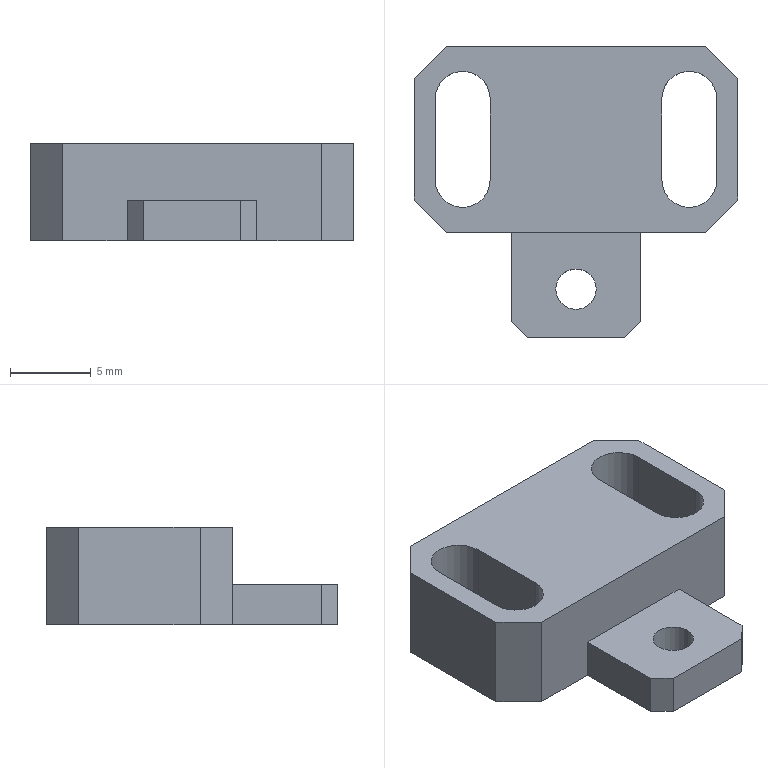Part | SolidWorks | features HoleWzd 3, Chamfer 2, ICE 2, Extrusion 1 | 1 solid | 26 faces | box 20 x 18 x 6 mm | volume 1134 mm3 | plane 20 | cylinder 6 | commonest cylinder face diameters 3.4 x4 2.5 x2
STEP:
#1=CARTESIAN_POINT('',(-1.25,-6.,0.));
#2=VERTEX_POINT('',#1);
#3=CARTESIAN_POINT('',(1.25,-6.,0.));
#4=VERTEX_POINT('',#3);
#5=CARTESIAN_POINT('',(0.,-6.,0.));
#6=DIRECTION('',(0.,0.,1.));
#7=DIRECTION('',(1.,0.,0.));
#8=AXIS2_PLACEMENT_3D('',#5,#6,#7);
#9=CIRCLE('',#8,1.25);
#10=EDGE_CURVE('',#2,#4,#9,.T.);
#11=ORIENTED_EDGE('',*,*,#10,.F.);
#12=CARTESIAN_POINT('',(-1.25,-6.,2.5));
#13=VERTEX_POINT('',#12);
#14=CARTESIAN_POINT('',(-1.25,-6.,6.));
#15=DIRECTION('',(0.,0.,1.));
#16=VECTOR('',#15,1000.);
#17=LINE('',#14,#16);
#18=EDGE_CURVE('',#2,#13,#17,.T.);
#19=ORIENTED_EDGE('',*,*,#18,.T.);
#20=CARTESIAN_POINT('',(1.25,-6.,2.5));
#21=VERTEX_POINT('',#20);
#22=CARTESIAN_POINT('',(0.,-6.,2.5));
#23=DIRECTION('',(0.,0.,-1.));
#24=DIRECTION('',(1.,0.,0.));
#25=AXIS2_PLACEMENT_3D('',#22,#23,#24);
#26=CIRCLE('',#25,1.25);
#27=EDGE_CURVE('',#21,#13,#26,.T.);
#28=ORIENTED_EDGE('',*,*,#27,.F.);
#29=CARTESIAN_POINT('',(1.25,-6.,6.));
#30=DIRECTION('',(0.,0.,1.));
#31=VECTOR('',#30,1000.);
#32=LINE('',#29,#31);
#33=EDGE_CURVE('',#4,#21,#32,.T.);
#34=ORIENTED_EDGE('',*,*,#33,.F.);
#35=EDGE_LOOP('',(#11,#19,#28,#34));
#36=FACE_OUTER_BOUND('',#35,.T.);
#37=CARTESIAN_POINT('',(0.,-6.,6.));
#38=DIRECTION('',(0.,0.,1.));
#39=DIRECTION('',(1.,0.,0.));
#40=AXIS2_PLACEMENT_3D('',#37,#38,#39);
#41=CYLINDRICAL_SURFACE('',#40,1.25);
#42=ADVANCED_FACE('',(#36),#41,.F.);
#43=CARTESIAN_POINT('',(-4.,-2.5,0.));
#44=VERTEX_POINT('',#43);
#45=CARTESIAN_POINT('',(-4.,-8.,0.));
#46=VERTEX_POINT('',#45);
#47=CARTESIAN_POINT('',(-4.,9.,0.));
#48=DIRECTION('',(0.,-1.,0.));
#49=VECTOR('',#48,1000.);
#50=LINE('',#47,#49);
#51=EDGE_CURVE('',#44,#46,#50,.T.);
#52=ORIENTED_EDGE('',*,*,#51,.T.);
#53=CARTESIAN_POINT('',(-4.,-8.,2.5));
#54=VERTEX_POINT('',#53);
#55=CARTESIAN_POINT('',(-4.,-8.,6.));
#56=DIRECTION('',(0.,0.,1.));
#57=VECTOR('',#56,1000.);
#58=LINE('',#55,#57);
#59=EDGE_CURVE('',#46,#54,#58,.T.);
#60=ORIENTED_EDGE('',*,*,#59,.T.);
#61=CARTESIAN_POINT('',(-4.,-2.5,2.5));
#62=VERTEX_POINT('',#61);
#63=CARTESIAN_POINT('',(-4.,-9.,2.5));
#64=DIRECTION('',(0.,1.,0.));
#65=VECTOR('',#64,1000.);
#66=LINE('',#63,#65);
#67=EDGE_CURVE('',#54,#62,#66,.T.);
#68=ORIENTED_EDGE('',*,*,#67,.T.);
#69=CARTESIAN_POINT('',(-4.,-2.5,-12.971));
#70=DIRECTION('',(0.,0.,1.));
#71=VECTOR('',#70,1000.);
#72=LINE('',#69,#71);
#73=EDGE_CURVE('',#44,#62,#72,.T.);
#74=ORIENTED_EDGE('',*,*,#73,.F.);
#75=EDGE_LOOP('',(#52,#60,#68,#74));
#76=FACE_OUTER_BOUND('',#75,.T.);
#77=CARTESIAN_POINT('',(-4.,9.,6.));
#78=DIRECTION('',(1.,0.,0.));
#79=DIRECTION('',(0.,1.,0.));
#80=AXIS2_PLACEMENT_3D('',#77,#78,#79);
#81=PLANE('',#80);
#82=ADVANCED_FACE('',(#76),#81,.F.);
#83=CARTESIAN_POINT('',(3.,-9.,2.5));
#84=VERTEX_POINT('',#83);
#85=CARTESIAN_POINT('',(-3.,-9.,2.5));
#86=VERTEX_POINT('',#85);
#87=CARTESIAN_POINT('',(-4.,-9.,2.5));
#88=DIRECTION('',(-1.,0.,0.));
#89=VECTOR('',#88,1000.);
#90=LINE('',#87,#89);
#91=EDGE_CURVE('',#84,#86,#90,.T.);
#92=ORIENTED_EDGE('',*,*,#91,.T.);
#93=CARTESIAN_POINT('',(-3.,-9.,0.));
#94=VERTEX_POINT('',#93);
#95=CARTESIAN_POINT('',(-3.,-9.,6.));
#96=DIRECTION('',(0.,0.,-1.));
#97=VECTOR('',#96,1000.);
#98=LINE('',#95,#97);
#99=EDGE_CURVE('',#86,#94,#98,.T.);
#100=ORIENTED_EDGE('',*,*,#99,.T.);
#101=CARTESIAN_POINT('',(3.,-9.,0.));
#102=VERTEX_POINT('',#101);
#103=CARTESIAN_POINT('',(-4.,-9.,0.));
#104=DIRECTION('',(1.,0.,0.));
#105=VECTOR('',#104,1000.);
#106=LINE('',#103,#105);
#107=EDGE_CURVE('',#94,#102,#106,.T.);
#108=ORIENTED_EDGE('',*,*,#107,.T.);
#109=CARTESIAN_POINT('',(3.,-9.,6.));
#110=DIRECTION('',(0.,0.,1.));
#111=VECTOR('',#110,1000.);
#112=LINE('',#109,#111);
#113=EDGE_CURVE('',#102,#84,#112,.T.);
#114=ORIENTED_EDGE('',*,*,#113,.T.);
#115=EDGE_LOOP('',(#92,#100,#108,#114));
#116=FACE_OUTER_BOUND('',#115,.T.);
#117=CARTESIAN_POINT('',(-4.,-9.,6.));
#118=DIRECTION('',(0.,1.,0.));
#119=DIRECTION('',(0.,0.,1.));
#120=AXIS2_PLACEMENT_3D('',#117,#118,#119);
#121=PLANE('',#120);
#122=ADVANCED_FACE('',(#116),#121,.F.);
#123=ORIENTED_EDGE('',*,*,#18,.F.);
#124=CARTESIAN_POINT('',(0.,-6.,0.));
#125=DIRECTION('',(0.,0.,1.));
#126=DIRECTION('',(1.,0.,0.));
#127=AXIS2_PLACEMENT_3D('',#124,#125,#126);
#128=CIRCLE('',#127,1.25);
#129=EDGE_CURVE('',#4,#2,#128,.T.);
#130=ORIENTED_EDGE('',*,*,#129,.F.);
#131=ORIENTED_EDGE('',*,*,#33,.T.);
#132=CARTESIAN_POINT('',(0.,-6.,2.5));
#133=DIRECTION('',(0.,0.,-1.));
#134=DIRECTION('',(1.,0.,0.));
#135=AXIS2_PLACEMENT_3D('',#132,#133,#134);
#136=CIRCLE('',#135,1.25);
#137=EDGE_CURVE('',#13,#21,#136,.T.);
#138=ORIENTED_EDGE('',*,*,#137,.F.);
#139=EDGE_LOOP('',(#123,#130,#131,#138));
#140=FACE_OUTER_BOUND('',#139,.T.);
#141=CARTESIAN_POINT('',(0.,-6.,6.));
#142=DIRECTION('',(0.,0.,1.));
#143=DIRECTION('',(1.,0.,0.));
#144=AXIS2_PLACEMENT_3D('',#141,#142,#143);
#145=CYLINDRICAL_SURFACE('',#144,1.25);
#146=ADVANCED_FACE('',(#140),#145,.F.);
#147=CARTESIAN_POINT('',(4.,-2.5,2.5));
#148=VERTEX_POINT('',#147);
#149=CARTESIAN_POINT('',(4.,-8.,2.5));
#150=VERTEX_POINT('',#149);
#151=CARTESIAN_POINT('',(4.,-9.,2.5));
#152=DIRECTION('',(0.,-1.,0.));
#153=VECTOR('',#152,1000.);
#154=LINE('',#151,#153);
#155=EDGE_CURVE('',#148,#150,#154,.T.);
#156=ORIENTED_EDGE('',*,*,#155,.T.);
#157=CARTESIAN_POINT('',(4.,-8.,0.));
#158=VERTEX_POINT('',#157);
#159=CARTESIAN_POINT('',(4.,-8.,6.));
#160=DIRECTION('',(0.,0.,-1.));
#161=VECTOR('',#160,1000.);
#162=LINE('',#159,#161);
#163=EDGE_CURVE('',#150,#158,#162,.T.);
#164=ORIENTED_EDGE('',*,*,#163,.T.);
#165=CARTESIAN_POINT('',(4.,-2.5,0.));
#166=VERTEX_POINT('',#165);
#167=CARTESIAN_POINT('',(4.,9.,0.));
#168=DIRECTION('',(0.,1.,0.));
#169=VECTOR('',#168,1000.);
#170=LINE('',#167,#169);
#171=EDGE_CURVE('',#158,#166,#170,.T.);
#172=ORIENTED_EDGE('',*,*,#171,.T.);
#173=CARTESIAN_POINT('',(4.,-2.5,-12.971));
#174=DIRECTION('',(0.,0.,1.));
#175=VECTOR('',#174,1000.);
#176=LINE('',#173,#175);
#177=EDGE_CURVE('',#166,#148,#176,.T.);
#178=ORIENTED_EDGE('',*,*,#177,.T.);
#179=EDGE_LOOP('',(#156,#164,#172,#178));
#180=FACE_OUTER_BOUND('',#179,.T.);
#181=CARTESIAN_POINT('',(4.,9.,6.));
#182=DIRECTION('',(-1.,0.,0.));
#183=DIRECTION('',(0.,-1.,0.));
#184=AXIS2_PLACEMENT_3D('',#181,#182,#183);
#185=PLANE('',#184);
#186=ADVANCED_FACE('',(#180),#185,.F.);
#187=CARTESIAN_POINT('',(8.,9.,6.));
#188=VERTEX_POINT('',#187);
#189=CARTESIAN_POINT('',(-8.,9.,6.));
#190=VERTEX_POINT('',#189);
#191=CARTESIAN_POINT('',(-4.,9.,6.));
#192=DIRECTION('',(-1.,0.,0.));
#193=VECTOR('',#192,1000.);
#194=LINE('',#191,#193);
#195=EDGE_CURVE('',#188,#190,#194,.T.);
#196=ORIENTED_EDGE('',*,*,#195,.F.);
#197=CARTESIAN_POINT('',(8.,9.,0.));
#198=VERTEX_POINT('',#197);
#199=CARTESIAN_POINT('',(8.,9.,0.));
#200=DIRECTION('',(0.,0.,-1.));
#201=VECTOR('',#200,1000.);
#202=LINE('',#199,#201);
#203=EDGE_CURVE('',#188,#198,#202,.T.);
#204=ORIENTED_EDGE('',*,*,#203,.T.);
#205=CARTESIAN_POINT('',(-8.,9.,0.));
#206=VERTEX_POINT('',#205);
#207=CARTESIAN_POINT('',(-4.,9.,0.));
#208=DIRECTION('',(-1.,0.,0.));
#209=VECTOR('',#208,1000.);
#210=LINE('',#207,#209);
#211=EDGE_CURVE('',#198,#206,#210,.T.);
#212=ORIENTED_EDGE('',*,*,#211,.T.);
#213=CARTESIAN_POINT('',(-8.,9.,6.));
#214=DIRECTION('',(0.,0.,1.));
#215=VECTOR('',#214,1000.);
#216=LINE('',#213,#215);
#217=EDGE_CURVE('',#206,#190,#216,.T.);
#218=ORIENTED_EDGE('',*,*,#217,.T.);
#219=EDGE_LOOP('',(#196,#204,#212,#218));
#220=FACE_OUTER_BOUND('',#219,.T.);
#221=CARTESIAN_POINT('',(-4.,9.,6.));
#222=DIRECTION('',(0.,-1.,0.));
#223=DIRECTION('',(0.,0.,-1.));
#224=AXIS2_PLACEMENT_3D('',#221,#222,#223);
#225=PLANE('',#224);
#226=ADVANCED_FACE('',(#220),#225,.F.);
#227=CARTESIAN_POINT('',(-5.3,5.75,6.));
#228=VERTEX_POINT('',#227);
#229=CARTESIAN_POINT('',(-8.7,5.75,6.));
#230=VERTEX_POINT('',#229);
#231=CARTESIAN_POINT('',(-7.,5.75,6.));
#232=DIRECTION('',(0.,0.,1.));
#233=DIRECTION('',(1.,0.,0.));
#234=AXIS2_PLACEMENT_3D('',#231,#232,#233);
#235=CIRCLE('',#234,1.7);
#236=EDGE_CURVE('',#228,#230,#235,.T.);
#237=ORIENTED_EDGE('',*,*,#236,.F.);
#238=CARTESIAN_POINT('',(-5.3,0.75,6.));
#239=VERTEX_POINT('',#238);
#240=CARTESIAN_POINT('',(-5.3,0.75,6.));
#241=DIRECTION('',(0.,1.,0.));
#242=VECTOR('',#241,1000.);
#243=LINE('',#240,#242);
#244=EDGE_CURVE('',#239,#228,#243,.T.);
#245=ORIENTED_EDGE('',*,*,#244,.F.);
#246=CARTESIAN_POINT('',(-8.7,0.75,6.));
#247=VERTEX_POINT('',#246);
#248=CARTESIAN_POINT('',(-7.,0.75,6.));
#249=DIRECTION('',(0.,0.,1.));
#250=DIRECTION('',(1.,0.,0.));
#251=AXIS2_PLACEMENT_3D('',#248,#249,#250);
#252=CIRCLE('',#251,1.7);
#253=EDGE_CURVE('',#247,#239,#252,.T.);
#254=ORIENTED_EDGE('',*,*,#253,.F.);
#255=CARTESIAN_POINT('',(-8.7,0.75,6.));
#256=DIRECTION('',(0.,1.,0.));
#257=VECTOR('',#256,1000.);
#258=LINE('',#255,#257);
#259=EDGE_CURVE('',#247,#230,#258,.T.);
#260=ORIENTED_EDGE('',*,*,#259,.T.);
#261=EDGE_LOOP('',(#237,#245,#254,#260));
#262=FACE_BOUND('',#261,.T.);
#263=CARTESIAN_POINT('',(8.7,5.75,6.));
#264=VERTEX_POINT('',#263);
#265=CARTESIAN_POINT('',(5.3,5.75,6.));
#266=VERTEX_POINT('',#265);
#267=CARTESIAN_POINT('',(7.,5.75,6.));
#268=DIRECTION('',(0.,0.,1.));
#269=DIRECTION('',(1.,0.,0.));
#270=AXIS2_PLACEMENT_3D('',#267,#268,#269);
#271=CIRCLE('',#270,1.7);
#272=EDGE_CURVE('',#264,#266,#271,.T.);
#273=ORIENTED_EDGE('',*,*,#272,.F.);
#274=CARTESIAN_POINT('',(8.7,0.75,6.));
#275=VERTEX_POINT('',#274);
#276=CARTESIAN_POINT('',(8.7,0.75,6.));
#277=DIRECTION('',(0.,1.,0.));
#278=VECTOR('',#277,1000.);
#279=LINE('',#276,#278);
#280=EDGE_CURVE('',#275,#264,#279,.T.);
#281=ORIENTED_EDGE('',*,*,#280,.F.);
#282=CARTESIAN_POINT('',(5.3,0.75,6.));
#283=VERTEX_POINT('',#282);
#284=CARTESIAN_POINT('',(7.,0.75,6.));
#285=DIRECTION('',(0.,0.,1.));
#286=DIRECTION('',(1.,0.,0.));
#287=AXIS2_PLACEMENT_3D('',#284,#285,#286);
#288=CIRCLE('',#287,1.7);
#289=EDGE_CURVE('',#283,#275,#288,.T.);
#290=ORIENTED_EDGE('',*,*,#289,.F.);
#291=CARTESIAN_POINT('',(5.3,0.75,6.));
#292=DIRECTION('',(0.,1.,0.));
#293=VECTOR('',#292,1000.);
#294=LINE('',#291,#293);
#295=EDGE_CURVE('',#283,#266,#294,.T.);
#296=ORIENTED_EDGE('',*,*,#295,.T.);
#297=EDGE_LOOP('',(#273,#281,#290,#296));
#298=FACE_BOUND('',#297,.T.);
#299=CARTESIAN_POINT('',(8.,-2.5,6.));
#300=VERTEX_POINT('',#299);
#301=CARTESIAN_POINT('',(-8.,-2.5,6.));
#302=VERTEX_POINT('',#301);
#303=CARTESIAN_POINT('',(-4.,-2.5,6.));
#304=DIRECTION('',(-1.,0.,0.));
#305=VECTOR('',#304,1000.);
#306=LINE('',#303,#305);
#307=EDGE_CURVE('',#300,#302,#306,.T.);
#308=ORIENTED_EDGE('',*,*,#307,.F.);
#309=CARTESIAN_POINT('',(10.,-0.5,6.));
#310=VERTEX_POINT('',#309);
#311=CARTESIAN_POINT('',(5.25,-5.25,6.));
#312=DIRECTION('',(0.7071,0.7071,0.));
#313=VECTOR('',#312,1000.);
#314=LINE('',#311,#313);
#315=EDGE_CURVE('',#300,#310,#314,.T.);
#316=ORIENTED_EDGE('',*,*,#315,.T.);
#317=CARTESIAN_POINT('',(10.,7.,6.));
#318=VERTEX_POINT('',#317);
#319=CARTESIAN_POINT('',(10.,9.,6.));
#320=DIRECTION('',(0.,1.,0.));
#321=VECTOR('',#320,1000.);
#322=LINE('',#319,#321);
#323=EDGE_CURVE('',#310,#318,#322,.T.);
#324=ORIENTED_EDGE('',*,*,#323,.T.);
#325=CARTESIAN_POINT('',(8.5,8.5,6.));
#326=DIRECTION('',(-0.7071,0.7071,0.));
#327=VECTOR('',#326,1000.);
#328=LINE('',#325,#327);
#329=EDGE_CURVE('',#318,#188,#328,.T.);
#330=ORIENTED_EDGE('',*,*,#329,.T.);
#331=ORIENTED_EDGE('',*,*,#195,.T.);
#332=CARTESIAN_POINT('',(-10.,7.,6.));
#333=VERTEX_POINT('',#332);
#334=CARTESIAN_POINT('',(-8.5,8.5,6.));
#335=DIRECTION('',(-0.7071,-0.7071,0.));
#336=VECTOR('',#335,1000.);
#337=LINE('',#334,#336);
#338=EDGE_CURVE('',#190,#333,#337,.T.);
#339=ORIENTED_EDGE('',*,*,#338,.T.);
#340=CARTESIAN_POINT('',(-10.,-0.5,6.));
#341=VERTEX_POINT('',#340);
#342=CARTESIAN_POINT('',(-10.,9.,6.));
#343=DIRECTION('',(0.,-1.,0.));
#344=VECTOR('',#343,1000.);
#345=LINE('',#342,#344);
#346=EDGE_CURVE('',#333,#341,#345,.T.);
#347=ORIENTED_EDGE('',*,*,#346,.T.);
#348=CARTESIAN_POINT('',(-5.25,-5.25,6.));
#349=DIRECTION('',(0.7071,-0.7071,0.));
#350=VECTOR('',#349,1000.);
#351=LINE('',#348,#350);
#352=EDGE_CURVE('',#341,#302,#351,.T.);
#353=ORIENTED_EDGE('',*,*,#352,.T.);
#354=EDGE_LOOP('',(#308,#316,#324,#330,#331,#339,#347,#353));
#355=FACE_OUTER_BOUND('',#354,.T.);
#356=CARTESIAN_POINT('',(0.,0.,6.));
#357=DIRECTION('',(0.,0.,1.));
#358=DIRECTION('',(1.,0.,0.));
#359=AXIS2_PLACEMENT_3D('',#356,#357,#358);
#360=PLANE('',#359);
#361=ADVANCED_FACE('',(#262,#298,#355),#360,.T.);
#362=CARTESIAN_POINT('',(-8.7,0.75,0.));
#363=VERTEX_POINT('',#362);
#364=CARTESIAN_POINT('',(-8.7,5.75,0.));
#365=VERTEX_POINT('',#364);
#366=CARTESIAN_POINT('',(-8.7,0.75,0.));
#367=DIRECTION('',(0.,1.,0.));
#368=VECTOR('',#367,1000.);
#369=LINE('',#366,#368);
#370=EDGE_CURVE('',#363,#365,#369,.T.);
#371=ORIENTED_EDGE('',*,*,#370,.F.);
#372=CARTESIAN_POINT('',(-5.3,0.75,0.));
#373=VERTEX_POINT('',#372);
#374=CARTESIAN_POINT('',(-7.,0.75,0.));
#375=DIRECTION('',(0.,0.,1.));
#376=DIRECTION('',(1.,0.,0.));
#377=AXIS2_PLACEMENT_3D('',#374,#375,#376);
#378=CIRCLE('',#377,1.7);
#379=EDGE_CURVE('',#363,#373,#378,.T.);
#380=ORIENTED_EDGE('',*,*,#379,.T.);
#381=CARTESIAN_POINT('',(-5.3,5.75,0.));
#382=VERTEX_POINT('',#381);
#383=CARTESIAN_POINT('',(-5.3,0.75,0.));
#384=DIRECTION('',(0.,1.,0.));
#385=VECTOR('',#384,1000.);
#386=LINE('',#383,#385);
#387=EDGE_CURVE('',#373,#382,#386,.T.);
#388=ORIENTED_EDGE('',*,*,#387,.T.);
#389=CARTESIAN_POINT('',(-7.,5.75,0.));
#390=DIRECTION('',(0.,0.,1.));
#391=DIRECTION('',(1.,0.,0.));
#392=AXIS2_PLACEMENT_3D('',#389,#390,#391);
#393=CIRCLE('',#392,1.7);
#394=EDGE_CURVE('',#382,#365,#393,.T.);
#395=ORIENTED_EDGE('',*,*,#394,.T.);
#396=EDGE_LOOP('',(#371,#380,#388,#395));
#397=FACE_BOUND('',#396,.T.);
#398=CARTESIAN_POINT('',(8.7,0.75,0.));
#399=VERTEX_POINT('',#398);
#400=CARTESIAN_POINT('',(8.7,5.75,0.));
#401=VERTEX_POINT('',#400);
#402=CARTESIAN_POINT('',(8.7,0.75,0.));
#403=DIRECTION('',(0.,1.,0.));
#404=VECTOR('',#403,1000.);
#405=LINE('',#402,#404);
#406=EDGE_CURVE('',#399,#401,#405,.T.);
#407=ORIENTED_EDGE('',*,*,#406,.T.);
#408=CARTESIAN_POINT('',(5.3,5.75,0.));
#409=VERTEX_POINT('',#408);
#410=CARTESIAN_POINT('',(7.,5.75,0.));
#411=DIRECTION('',(0.,0.,1.));
#412=DIRECTION('',(1.,0.,0.));
#413=AXIS2_PLACEMENT_3D('',#410,#411,#412);
#414=CIRCLE('',#413,1.7);
#415=EDGE_CURVE('',#401,#409,#414,.T.);
#416=ORIENTED_EDGE('',*,*,#415,.T.);
#417=CARTESIAN_POINT('',(5.3,0.75,0.));
#418=VERTEX_POINT('',#417);
#419=CARTESIAN_POINT('',(5.3,0.75,0.));
#420=DIRECTION('',(0.,1.,0.));
#421=VECTOR('',#420,1000.);
#422=LINE('',#419,#421);
#423=EDGE_CURVE('',#418,#409,#422,.T.);
#424=ORIENTED_EDGE('',*,*,#423,.F.);
#425=CARTESIAN_POINT('',(7.,0.75,0.));
#426=DIRECTION('',(0.,0.,1.));
#427=DIRECTION('',(1.,0.,0.));
#428=AXIS2_PLACEMENT_3D('',#425,#426,#427);
#429=CIRCLE('',#428,1.7);
#430=EDGE_CURVE('',#418,#399,#429,.T.);
#431=ORIENTED_EDGE('',*,*,#430,.T.);
#432=EDGE_LOOP('',(#407,#416,#424,#431));
#433=FACE_BOUND('',#432,.T.);
#434=ORIENTED_EDGE('',*,*,#129,.T.);
#435=ORIENTED_EDGE('',*,*,#10,.T.);
#436=EDGE_LOOP('',(#434,#435));
#437=FACE_BOUND('',#436,.T.);
#438=ORIENTED_EDGE('',*,*,#107,.F.);
#439=CARTESIAN_POINT('',(-3.,-9.,0.));
#440=DIRECTION('',(-0.7071,0.7071,0.));
#441=VECTOR('',#440,1000.);
#442=LINE('',#439,#441);
#443=EDGE_CURVE('',#94,#46,#442,.T.);
#444=ORIENTED_EDGE('',*,*,#443,.T.);
#445=ORIENTED_EDGE('',*,*,#51,.F.);
#446=CARTESIAN_POINT('',(-8.,-2.5,0.));
#447=VERTEX_POINT('',#446);
#448=CARTESIAN_POINT('',(-4.,-2.5,0.));
#449=DIRECTION('',(-1.,0.,0.));
#450=VECTOR('',#449,1000.);
#451=LINE('',#448,#450);
#452=EDGE_CURVE('',#44,#447,#451,.T.);
#453=ORIENTED_EDGE('',*,*,#452,.T.);
#454=CARTESIAN_POINT('',(-10.,-0.5,0.));
#455=VERTEX_POINT('',#454);
#456=CARTESIAN_POINT('',(-10.,-0.5,0.));
#457=DIRECTION('',(-0.7071,0.7071,0.));
#458=VECTOR('',#457,1000.);
#459=LINE('',#456,#458);
#460=EDGE_CURVE('',#447,#455,#459,.T.);
#461=ORIENTED_EDGE('',*,*,#460,.T.);
#462=CARTESIAN_POINT('',(-10.,7.,0.));
#463=VERTEX_POINT('',#462);
#464=CARTESIAN_POINT('',(-10.,9.,0.));
#465=DIRECTION('',(0.,1.,0.));
#466=VECTOR('',#465,1000.);
#467=LINE('',#464,#466);
#468=EDGE_CURVE('',#455,#463,#467,.T.);
#469=ORIENTED_EDGE('',*,*,#468,.T.);
#470=CARTESIAN_POINT('',(-8.,9.,0.));
#471=DIRECTION('',(0.7071,0.7071,0.));
#472=VECTOR('',#471,1000.);
#473=LINE('',#470,#472);
#474=EDGE_CURVE('',#463,#206,#473,.T.);
#475=ORIENTED_EDGE('',*,*,#474,.T.);
#476=ORIENTED_EDGE('',*,*,#211,.F.);
#477=CARTESIAN_POINT('',(10.,7.,0.));
#478=VERTEX_POINT('',#477);
#479=CARTESIAN_POINT('',(10.,7.,0.));
#480=DIRECTION('',(0.7071,-0.7071,0.));
#481=VECTOR('',#480,1000.);
#482=LINE('',#479,#481);
#483=EDGE_CURVE('',#198,#478,#482,.T.);
#484=ORIENTED_EDGE('',*,*,#483,.T.);
#485=CARTESIAN_POINT('',(10.,-0.5,0.));
#486=VERTEX_POINT('',#485);
#487=CARTESIAN_POINT('',(10.,9.,0.));
#488=DIRECTION('',(0.,-1.,0.));
#489=VECTOR('',#488,1000.);
#490=LINE('',#487,#489);
#491=EDGE_CURVE('',#478,#486,#490,.T.);
#492=ORIENTED_EDGE('',*,*,#491,.T.);
#493=CARTESIAN_POINT('',(8.,-2.5,0.));
#494=VERTEX_POINT('',#493);
#495=CARTESIAN_POINT('',(8.,-2.5,0.));
#496=DIRECTION('',(-0.7071,-0.7071,0.));
#497=VECTOR('',#496,1000.);
#498=LINE('',#495,#497);
#499=EDGE_CURVE('',#486,#494,#498,.T.);
#500=ORIENTED_EDGE('',*,*,#499,.T.);
#501=CARTESIAN_POINT('',(4.,-2.5,0.));
#502=DIRECTION('',(-1.,0.,0.));
#503=VECTOR('',#502,1000.);
#504=LINE('',#501,#503);
#505=EDGE_CURVE('',#494,#166,#504,.T.);
#506=ORIENTED_EDGE('',*,*,#505,.T.);
#507=ORIENTED_EDGE('',*,*,#171,.F.);
#508=CARTESIAN_POINT('',(4.,-8.,0.));
#509=DIRECTION('',(-0.7071,-0.7071,0.));
#510=VECTOR('',#509,1000.);
#511=LINE('',#508,#510);
#512=EDGE_CURVE('',#158,#102,#511,.T.);
#513=ORIENTED_EDGE('',*,*,#512,.T.);
#514=EDGE_LOOP('',(#438,#444,#445,#453,#461,#469,#475,#476,#484,#492,#500,#506,#507,#513));
#515=FACE_OUTER_BOUND('',#514,.T.);
#516=CARTESIAN_POINT('',(0.,0.,0.));
#517=DIRECTION('',(0.,0.,1.));
#518=DIRECTION('',(1.,0.,0.));
#519=AXIS2_PLACEMENT_3D('',#516,#517,#518);
#520=PLANE('',#519);
#521=ADVANCED_FACE('',(#397,#433,#437,#515),#520,.F.);
#522=ORIENTED_EDGE('',*,*,#67,.F.);
#523=CARTESIAN_POINT('',(-6.,-6.,2.5));
#524=DIRECTION('',(0.7071,-0.7071,0.));
#525=VECTOR('',#524,1000.);
#526=LINE('',#523,#525);
#527=EDGE_CURVE('',#54,#86,#526,.T.);
#528=ORIENTED_EDGE('',*,*,#527,.T.);
#529=ORIENTED_EDGE('',*,*,#91,.F.);
#530=CARTESIAN_POINT('',(6.,-6.,2.5));
#531=DIRECTION('',(0.7071,0.7071,0.));
#532=VECTOR('',#531,1000.);
#533=LINE('',#530,#532);
#534=EDGE_CURVE('',#84,#150,#533,.T.);
#535=ORIENTED_EDGE('',*,*,#534,.T.);
#536=ORIENTED_EDGE('',*,*,#155,.F.);
#537=CARTESIAN_POINT('',(-4.,-2.5,2.5));
#538=DIRECTION('',(1.,0.,0.));
#539=VECTOR('',#538,1000.);
#540=LINE('',#537,#539);
#541=EDGE_CURVE('',#62,#148,#540,.T.);
#542=ORIENTED_EDGE('',*,*,#541,.F.);
#543=EDGE_LOOP('',(#522,#528,#529,#535,#536,#542));
#544=FACE_OUTER_BOUND('',#543,.T.);
#545=ORIENTED_EDGE('',*,*,#27,.T.);
#546=ORIENTED_EDGE('',*,*,#137,.T.);
#547=EDGE_LOOP('',(#545,#546));
#548=FACE_BOUND('',#547,.T.);
#549=CARTESIAN_POINT('',(0.,0.,2.5));
#550=DIRECTION('',(0.,0.,1.));
#551=DIRECTION('',(1.,0.,0.));
#552=AXIS2_PLACEMENT_3D('',#549,#550,#551);
#553=PLANE('',#552);
#554=ADVANCED_FACE('',(#544,#548),#553,.T.);
#555=ORIENTED_EDGE('',*,*,#505,.F.);
#556=CARTESIAN_POINT('',(8.,-2.5,6.));
#557=DIRECTION('',(0.,0.,1.));
#558=VECTOR('',#557,1000.);
#559=LINE('',#556,#558);
#560=EDGE_CURVE('',#494,#300,#559,.T.);
#561=ORIENTED_EDGE('',*,*,#560,.T.);
#562=ORIENTED_EDGE('',*,*,#307,.T.);
#563=CARTESIAN_POINT('',(-8.,-2.5,0.));
#564=DIRECTION('',(0.,0.,-1.));
#565=VECTOR('',#564,1000.);
#566=LINE('',#563,#565);
#567=EDGE_CURVE('',#302,#447,#566,.T.);
#568=ORIENTED_EDGE('',*,*,#567,.T.);
#569=ORIENTED_EDGE('',*,*,#452,.F.);
#570=ORIENTED_EDGE('',*,*,#73,.T.);
#571=ORIENTED_EDGE('',*,*,#541,.T.);
#572=ORIENTED_EDGE('',*,*,#177,.F.);
#573=EDGE_LOOP('',(#555,#561,#562,#568,#569,#570,#571,#572));
#574=FACE_OUTER_BOUND('',#573,.T.);
#575=CARTESIAN_POINT('',(-4.,-2.5,-10.308));
#576=DIRECTION('',(0.,1.,0.));
#577=DIRECTION('',(0.,0.,1.));
#578=AXIS2_PLACEMENT_3D('',#575,#576,#577);
#579=PLANE('',#578);
#580=ADVANCED_FACE('',(#574),#579,.F.);
#581=ORIENTED_EDGE('',*,*,#346,.F.);
#582=CARTESIAN_POINT('',(-10.,7.,0.));
#583=DIRECTION('',(0.,0.,-1.));
#584=VECTOR('',#583,1000.);
#585=LINE('',#582,#584);
#586=EDGE_CURVE('',#333,#463,#585,.T.);
#587=ORIENTED_EDGE('',*,*,#586,.T.);
#588=ORIENTED_EDGE('',*,*,#468,.F.);
#589=CARTESIAN_POINT('',(-10.,-0.5,6.));
#590=DIRECTION('',(0.,0.,1.));
#591=VECTOR('',#590,1000.);
#592=LINE('',#589,#591);
#593=EDGE_CURVE('',#455,#341,#592,.T.);
#594=ORIENTED_EDGE('',*,*,#593,.T.);
#595=EDGE_LOOP('',(#581,#587,#588,#594));
#596=FACE_OUTER_BOUND('',#595,.T.);
#597=CARTESIAN_POINT('',(-10.,9.,-12.971));
#598=DIRECTION('',(-1.,0.,0.));
#599=DIRECTION('',(0.,-1.,0.));
#600=AXIS2_PLACEMENT_3D('',#597,#598,#599);
#601=PLANE('',#600);
#602=ADVANCED_FACE('',(#596),#601,.T.);
#603=ORIENTED_EDGE('',*,*,#323,.F.);
#604=CARTESIAN_POINT('',(10.,-0.5,0.));
#605=DIRECTION('',(0.,0.,-1.));
#606=VECTOR('',#605,1000.);
#607=LINE('',#604,#606);
#608=EDGE_CURVE('',#310,#486,#607,.T.);
#609=ORIENTED_EDGE('',*,*,#608,.T.);
#610=ORIENTED_EDGE('',*,*,#491,.F.);
#611=CARTESIAN_POINT('',(10.,7.,6.));
#612=DIRECTION('',(0.,0.,1.));
#613=VECTOR('',#612,1000.);
#614=LINE('',#611,#613);
#615=EDGE_CURVE('',#478,#318,#614,.T.);
#616=ORIENTED_EDGE('',*,*,#615,.T.);
#617=EDGE_LOOP('',(#603,#609,#610,#616));
#618=FACE_OUTER_BOUND('',#617,.T.);
#619=CARTESIAN_POINT('',(10.,9.,-12.971));
#620=DIRECTION('',(1.,0.,0.));
#621=DIRECTION('',(0.,1.,0.));
#622=AXIS2_PLACEMENT_3D('',#619,#620,#621);
#623=PLANE('',#622);
#624=ADVANCED_FACE('',(#618),#623,.T.);
#625=ORIENTED_EDGE('',*,*,#415,.F.);
#626=CARTESIAN_POINT('',(8.7,5.75,0.));
#627=DIRECTION('',(0.,0.,-1.));
#628=VECTOR('',#627,1000.);
#629=LINE('',#626,#628);
#630=EDGE_CURVE('',#264,#401,#629,.T.);
#631=ORIENTED_EDGE('',*,*,#630,.F.);
#632=ORIENTED_EDGE('',*,*,#272,.T.);
#633=CARTESIAN_POINT('',(5.3,5.75,6.));
#634=DIRECTION('',(0.,0.,1.));
#635=VECTOR('',#634,1000.);
#636=LINE('',#633,#635);
#637=EDGE_CURVE('',#409,#266,#636,.T.);
#638=ORIENTED_EDGE('',*,*,#637,.F.);
#639=EDGE_LOOP('',(#625,#631,#632,#638));
#640=FACE_OUTER_BOUND('',#639,.T.);
#641=CARTESIAN_POINT('',(7.,5.75,6.));
#642=DIRECTION('',(0.,0.,1.));
#643=DIRECTION('',(1.,0.,0.));
#644=AXIS2_PLACEMENT_3D('',#641,#642,#643);
#645=CYLINDRICAL_SURFACE('',#644,1.7);
#646=ADVANCED_FACE('',(#640),#645,.F.);
#647=ORIENTED_EDGE('',*,*,#289,.T.);
#648=CARTESIAN_POINT('',(8.7,0.75,0.));
#649=DIRECTION('',(0.,0.,-1.));
#650=VECTOR('',#649,1000.);
#651=LINE('',#648,#650);
#652=EDGE_CURVE('',#275,#399,#651,.T.);
#653=ORIENTED_EDGE('',*,*,#652,.T.);
#654=ORIENTED_EDGE('',*,*,#430,.F.);
#655=CARTESIAN_POINT('',(5.3,0.75,6.));
#656=DIRECTION('',(0.,0.,-1.));
#657=VECTOR('',#656,1000.);
#658=LINE('',#655,#657);
#659=EDGE_CURVE('',#283,#418,#658,.T.);
#660=ORIENTED_EDGE('',*,*,#659,.F.);
#661=EDGE_LOOP('',(#647,#653,#654,#660));
#662=FACE_OUTER_BOUND('',#661,.T.);
#663=CARTESIAN_POINT('',(7.,0.75,6.));
#664=DIRECTION('',(0.,0.,1.));
#665=DIRECTION('',(1.,0.,0.));
#666=AXIS2_PLACEMENT_3D('',#663,#664,#665);
#667=CYLINDRICAL_SURFACE('',#666,1.7);
#668=ADVANCED_FACE('',(#662),#667,.F.);
#669=ORIENTED_EDGE('',*,*,#637,.T.);
#670=ORIENTED_EDGE('',*,*,#295,.F.);
#671=ORIENTED_EDGE('',*,*,#659,.T.);
#672=ORIENTED_EDGE('',*,*,#423,.T.);
#673=EDGE_LOOP('',(#669,#670,#671,#672));
#674=FACE_OUTER_BOUND('',#673,.T.);
#675=CARTESIAN_POINT('',(5.3,0.75,6.));
#676=DIRECTION('',(-1.,0.,0.));
#677=DIRECTION('',(0.,0.,1.));
#678=AXIS2_PLACEMENT_3D('',#675,#676,#677);
#679=PLANE('',#678);
#680=ADVANCED_FACE('',(#674),#679,.F.);
#681=ORIENTED_EDGE('',*,*,#630,.T.);
#682=ORIENTED_EDGE('',*,*,#406,.F.);
#683=ORIENTED_EDGE('',*,*,#652,.F.);
#684=ORIENTED_EDGE('',*,*,#280,.T.);
#685=EDGE_LOOP('',(#681,#682,#683,#684));
#686=FACE_OUTER_BOUND('',#685,.T.);
#687=CARTESIAN_POINT('',(8.7,0.75,0.));
#688=DIRECTION('',(1.,0.,0.));
#689=DIRECTION('',(0.,0.,-1.));
#690=AXIS2_PLACEMENT_3D('',#687,#688,#689);
#691=PLANE('',#690);
#692=ADVANCED_FACE('',(#686),#691,.F.);
#693=ORIENTED_EDGE('',*,*,#394,.F.);
#694=CARTESIAN_POINT('',(-5.3,5.75,0.));
#695=DIRECTION('',(0.,0.,-1.));
#696=VECTOR('',#695,1000.);
#697=LINE('',#694,#696);
#698=EDGE_CURVE('',#228,#382,#697,.T.);
#699=ORIENTED_EDGE('',*,*,#698,.F.);
#700=ORIENTED_EDGE('',*,*,#236,.T.);
#701=CARTESIAN_POINT('',(-8.7,5.75,6.));
#702=DIRECTION('',(0.,0.,1.));
#703=VECTOR('',#702,1000.);
#704=LINE('',#701,#703);
#705=EDGE_CURVE('',#365,#230,#704,.T.);
#706=ORIENTED_EDGE('',*,*,#705,.F.);
#707=EDGE_LOOP('',(#693,#699,#700,#706));
#708=FACE_OUTER_BOUND('',#707,.T.);
#709=CARTESIAN_POINT('',(-7.,5.75,6.));
#710=DIRECTION('',(0.,0.,1.));
#711=DIRECTION('',(1.,0.,0.));
#712=AXIS2_PLACEMENT_3D('',#709,#710,#711);
#713=CYLINDRICAL_SURFACE('',#712,1.7);
#714=ADVANCED_FACE('',(#708),#713,.F.);
#715=ORIENTED_EDGE('',*,*,#253,.T.);
#716=CARTESIAN_POINT('',(-5.3,0.75,0.));
#717=DIRECTION('',(0.,0.,-1.));
#718=VECTOR('',#717,1000.);
#719=LINE('',#716,#718);
#720=EDGE_CURVE('',#239,#373,#719,.T.);
#721=ORIENTED_EDGE('',*,*,#720,.T.);
#722=ORIENTED_EDGE('',*,*,#379,.F.);
#723=CARTESIAN_POINT('',(-8.7,0.75,6.));
#724=DIRECTION('',(0.,0.,-1.));
#725=VECTOR('',#724,1000.);
#726=LINE('',#723,#725);
#727=EDGE_CURVE('',#247,#363,#726,.T.);
#728=ORIENTED_EDGE('',*,*,#727,.F.);
#729=EDGE_LOOP('',(#715,#721,#722,#728));
#730=FACE_OUTER_BOUND('',#729,.T.);
#731=CARTESIAN_POINT('',(-7.,0.75,6.));
#732=DIRECTION('',(0.,0.,1.));
#733=DIRECTION('',(1.,0.,0.));
#734=AXIS2_PLACEMENT_3D('',#731,#732,#733);
#735=CYLINDRICAL_SURFACE('',#734,1.7);
#736=ADVANCED_FACE('',(#730),#735,.F.);
#737=ORIENTED_EDGE('',*,*,#705,.T.);
#738=ORIENTED_EDGE('',*,*,#259,.F.);
#739=ORIENTED_EDGE('',*,*,#727,.T.);
#740=ORIENTED_EDGE('',*,*,#370,.T.);
#741=EDGE_LOOP('',(#737,#738,#739,#740));
#742=FACE_OUTER_BOUND('',#741,.T.);
#743=CARTESIAN_POINT('',(-8.7,0.75,6.));
#744=DIRECTION('',(-1.,0.,0.));
#745=DIRECTION('',(0.,0.,1.));
#746=AXIS2_PLACEMENT_3D('',#743,#744,#745);
#747=PLANE('',#746);
#748=ADVANCED_FACE('',(#742),#747,.F.);
#749=ORIENTED_EDGE('',*,*,#698,.T.);
#750=ORIENTED_EDGE('',*,*,#387,.F.);
#751=ORIENTED_EDGE('',*,*,#720,.F.);
#752=ORIENTED_EDGE('',*,*,#244,.T.);
#753=EDGE_LOOP('',(#749,#750,#751,#752));
#754=FACE_OUTER_BOUND('',#753,.T.);
#755=CARTESIAN_POINT('',(-5.3,0.75,0.));
#756=DIRECTION('',(1.,0.,0.));
#757=DIRECTION('',(0.,0.,-1.));
#758=AXIS2_PLACEMENT_3D('',#755,#756,#757);
#759=PLANE('',#758);
#760=ADVANCED_FACE('',(#754),#759,.F.);
#761=ORIENTED_EDGE('',*,*,#499,.F.);
#762=ORIENTED_EDGE('',*,*,#608,.F.);
#763=ORIENTED_EDGE('',*,*,#315,.F.);
#764=ORIENTED_EDGE('',*,*,#560,.F.);
#765=EDGE_LOOP('',(#761,#762,#763,#764));
#766=FACE_OUTER_BOUND('',#765,.T.);
#767=CARTESIAN_POINT('',(8.,-2.5,-10.308));
#768=DIRECTION('',(0.7071,-0.7071,0.));
#769=DIRECTION('',(0.,0.,-1.));
#770=AXIS2_PLACEMENT_3D('',#767,#768,#769);
#771=PLANE('',#770);
#772=ADVANCED_FACE('',(#766),#771,.T.);
#773=ORIENTED_EDGE('',*,*,#483,.F.);
#774=ORIENTED_EDGE('',*,*,#203,.F.);
#775=ORIENTED_EDGE('',*,*,#329,.F.);
#776=ORIENTED_EDGE('',*,*,#615,.F.);
#777=EDGE_LOOP('',(#773,#774,#775,#776));
#778=FACE_OUTER_BOUND('',#777,.T.);
#779=CARTESIAN_POINT('',(10.,7.,-12.971));
#780=DIRECTION('',(0.7071,0.7071,0.));
#781=DIRECTION('',(0.,0.,-1.));
#782=AXIS2_PLACEMENT_3D('',#779,#780,#781);
#783=PLANE('',#782);
#784=ADVANCED_FACE('',(#778),#783,.T.);
#785=ORIENTED_EDGE('',*,*,#474,.F.);
#786=ORIENTED_EDGE('',*,*,#586,.F.);
#787=ORIENTED_EDGE('',*,*,#338,.F.);
#788=ORIENTED_EDGE('',*,*,#217,.F.);
#789=EDGE_LOOP('',(#785,#786,#787,#788));
#790=FACE_OUTER_BOUND('',#789,.T.);
#791=CARTESIAN_POINT('',(-8.,9.,6.));
#792=DIRECTION('',(-0.7071,0.7071,0.));
#793=DIRECTION('',(0.,0.,-1.));
#794=AXIS2_PLACEMENT_3D('',#791,#792,#793);
#795=PLANE('',#794);
#796=ADVANCED_FACE('',(#790),#795,.T.);
#797=ORIENTED_EDGE('',*,*,#460,.F.);
#798=ORIENTED_EDGE('',*,*,#567,.F.);
#799=ORIENTED_EDGE('',*,*,#352,.F.);
#800=ORIENTED_EDGE('',*,*,#593,.F.);
#801=EDGE_LOOP('',(#797,#798,#799,#800));
#802=FACE_OUTER_BOUND('',#801,.T.);
#803=CARTESIAN_POINT('',(-10.,-0.5,-12.971));
#804=DIRECTION('',(-0.7071,-0.7071,0.));
#805=DIRECTION('',(0.,0.,-1.));
#806=AXIS2_PLACEMENT_3D('',#803,#804,#805);
#807=PLANE('',#806);
#808=ADVANCED_FACE('',(#802),#807,.T.);
#809=ORIENTED_EDGE('',*,*,#527,.F.);
#810=ORIENTED_EDGE('',*,*,#59,.F.);
#811=ORIENTED_EDGE('',*,*,#443,.F.);
#812=ORIENTED_EDGE('',*,*,#99,.F.);
#813=EDGE_LOOP('',(#809,#810,#811,#812));
#814=FACE_OUTER_BOUND('',#813,.T.);
#815=CARTESIAN_POINT('',(-3.,-9.,6.));
#816=DIRECTION('',(0.7071,0.7071,0.));
#817=DIRECTION('',(0.,0.,-1.));
#818=AXIS2_PLACEMENT_3D('',#815,#816,#817);
#819=PLANE('',#818);
#820=ADVANCED_FACE('',(#814),#819,.F.);
#821=ORIENTED_EDGE('',*,*,#534,.F.);
#822=ORIENTED_EDGE('',*,*,#113,.F.);
#823=ORIENTED_EDGE('',*,*,#512,.F.);
#824=ORIENTED_EDGE('',*,*,#163,.F.);
#825=EDGE_LOOP('',(#821,#822,#823,#824));
#826=FACE_OUTER_BOUND('',#825,.T.);
#827=CARTESIAN_POINT('',(4.,-8.,6.));
#828=DIRECTION('',(-0.7071,0.7071,0.));
#829=DIRECTION('',(0.,0.,-1.));
#830=AXIS2_PLACEMENT_3D('',#827,#828,#829);
#831=PLANE('',#830);
#832=ADVANCED_FACE('',(#826),#831,.F.);
#833=CLOSED_SHELL('',(#42,#82,#122,#146,#186,#226,#361,#521,#554,#580,#602,#624,#646,#668,#680,#692,#714,#736,#748,#760,#772,#784,#796,#808,#820,#832));
#834=MANIFOLD_SOLID_BREP('',#833);
#835=CARTESIAN_POINT('',(0.,0.,0.));
#836=DIRECTION('',(0.,0.,1.));
#837=DIRECTION('',(1.,0.,0.));
#838=AXIS2_PLACEMENT_3D('',#835,#836,#837);
#839=(LENGTH_UNIT()NAMED_UNIT(*)SI_UNIT(.MILLI.,.METRE.));
#840=UNCERTAINTY_MEASURE_WITH_UNIT(LENGTH_MEASURE(0.00001),#839,'','');
#841=(NAMED_UNIT(*)PLANE_ANGLE_UNIT()SI_UNIT($,.RADIAN.));
#842=(NAMED_UNIT(*)SI_UNIT($,.STERADIAN.)SOLID_ANGLE_UNIT());
#843=(GEOMETRIC_REPRESENTATION_CONTEXT(3)GLOBAL_UNCERTAINTY_ASSIGNED_CONTEXT((#840))GLOBAL_UNIT_ASSIGNED_CONTEXT((#839,#841,#842))REPRESENTATION_CONTEXT('',''));
#844=ADVANCED_BREP_SHAPE_REPRESENTATION('',(#834,#838),#843);